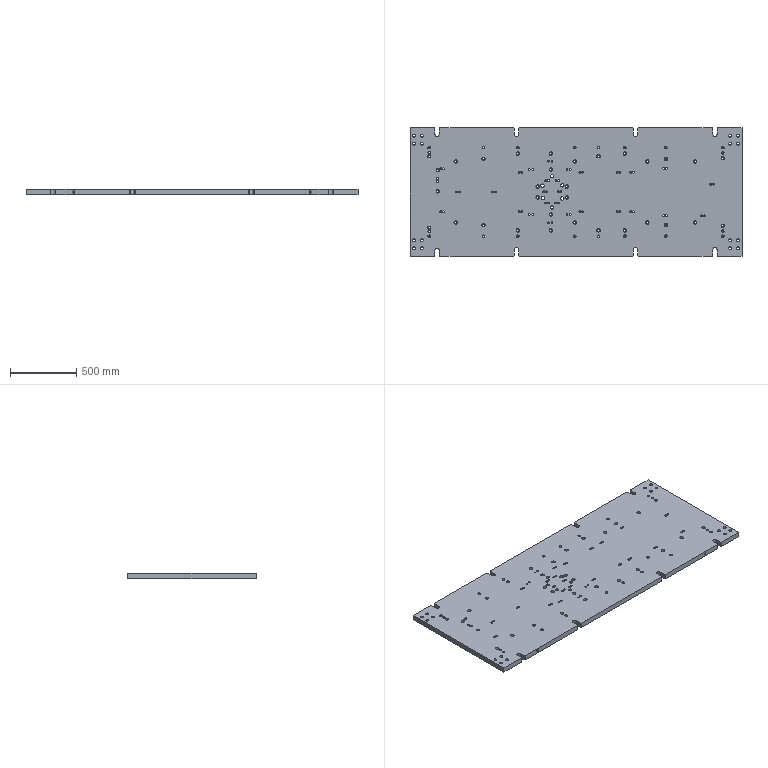Part | STEP file | 001_id2254_x_t | 1 solid | 362 faces | box 2510 x 970 x 40 mm | volume 95269879 mm3 | cylinder 228 | plane 98 | cone 36 | commonest cylinder face diameters 15 x44 26 x38 6.8 x32 17 x32 13 x16 20 x16